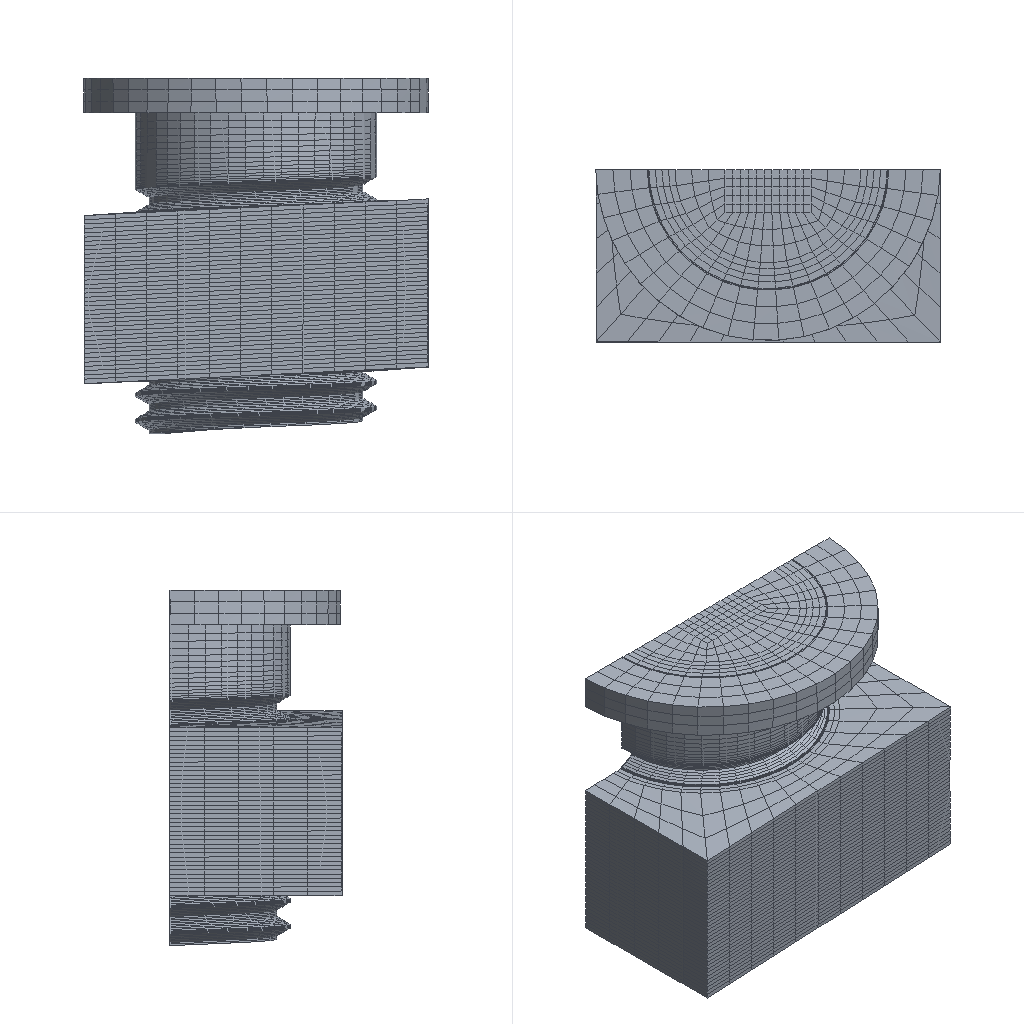Simulation study | abaqus
Set-up summary:
category,name,step,type,value,unit,region
solver,abaqus,,Abaqus/CAE 2024
units,mm-N-s-tonne (MPa),,inferred,E=213000 density=7.87e-09
analysis,Step-1,,dynamic implicit,time_period=1
mesh,nodes,,,41508
mesh,elements,,,35268
element_type,C3D8I,,,35268
material,MATERIAL-35CRMN,,E,213000
material,MATERIAL-35CRMN,,nu,0.286
material,MATERIAL-35CRMN,,density,7.87e-09
material,MATERIAL-35CRMN,,yield,480
material,MATERIAL-35CRMN,,behaviors,plastic
material,MATERIAL-45,,E,209000
material,MATERIAL-45,,nu,0.269
material,MATERIAL-45,,density,7.85e-09
material,MATERIAL-45,,yield,400
material,MATERIAL-45,,behaviors,plastic
section,MATERIAL-45,,solid section,,,NUT
section,MATERIAL-35CRMN,,solid section,,,BOLT
load,SURFFORCE-1,Step-1,pressure,50,,SUR_ELEMS
bc,Disp-BC-1,Step-1,fixed,[dofs=y],,SET-NODE-SYM-Y
bc,Disp-BC-2,Step-1,fixed,[dofs=rx],,SET-NODE-SYM-Y
bc,Disp-BC-3,Step-1,fixed,[dofs=rz],,SET-NODE-SYM-Y
bc,Disp-BC-4,Step-1,fixed,"[dofs=rx,ry,rz,x,y,z n=6]",,SET-NODE-FIX
contact,INTER1-1,initial,contact pair surface to surface,interaction=INTER1; friction=0.15,,SUR_S1 / SUR_M1
Abaqus input file, long lists of numbers shortened:
*Heading
** Job name: deck Model name: Thread
** Generated by: Abaqus/CAE 2024
*Preprint, echo=NO, model=NO, history=NO, contact=NO
**
** PARTS
**
*Part, name=PART-1
*Node
      1,  -6.295, -0.01523,   39.886
      2,  -6.245, -0.01539,    39.75
** (41506 more lines like these left out)
*Element, type=C3D8I
    1,   122,   115,   213,   212,  2308,  2309,  2310,  2311
    2,  2308,  2309,  2310,  2311,  2312,  2313,  2314,  2315
** (35266 more lines like these left out)
*Elset, elset=BOLT, generate
 11194,  35268,      1
*Elset, elset=NUT, generate
     1,  11193,      1
** Section: Section-1-NUT
*Solid Section, elset=NUT, material=MATERIAL-45
,
** Section: Section-2-BOLT
*Solid Section, elset=BOLT, material=MATERIAL-35CRMN
,
*End Part
**
**
** ASSEMBLY
**
*Assembly, name=Assembly
**
*Instance, name=PART-1-1, part=PART-1
*End Instance
**
*Elset, elset=SET-ELEMS, instance=PART-1-1
 26231, 26232, 26234, 26235, 26237, 26238, 26240, 26241, 26243, 26244, 26246, 26247, 26249, 26250, 26252, 26253
 26255, 26256, 26258, 26259, 26261, 26262, 26264, 26265, 26267, 26268, 26270, 26271, 26273, 26274, 26276, 26277
** (6 more lines like these left out)
*Nset, nset=SET-NODE-FIX, instance=PART-1-1
     7,     9,    10,    11,    12,    19,    20,    21,    22,    23,    24,    26,    27,    28,    31,    35
    42,    44,    45,    46,    55,    58,    63,    69,  1067,  1072,  1073,  1077,  1080,  1083,  1085,  1086
** (53 more lines like these left out)
*Nset, nset=SET-NODE-SYM-Y, instance=PART-1-1
     1,     2,     3,     4,    46,    48,    60,    64,    71,    72,    73,    74,    75,    76,    77,    78
    79,    80,    81,    82,    83,    84,    85,    86,    87,    88,    89,    90,    91,    92,    93,    94
** (260 more lines like these left out)
*Elset, elset=_SUR_ELEMS_S3, internal, instance=PART-1-1
 26231, 26232, 26234, 26235, 26237, 26238, 26240, 26241, 26243, 26244, 26246, 26247, 26249, 26250, 26252, 26253
 26255, 26256, 26258, 26259, 26261, 26262, 26264, 26265, 26267, 26268, 26270, 26271, 26273, 26274, 26276, 26277
** (6 more lines like these left out)
*Surface, type=ELEMENT, name=SUR_ELEMS
_SUR_ELEMS_S3, S3
*Elset, elset=_SUR_M1_S3, internal, instance=PART-1-1
 12139, 12140, 12141, 12142, 12143, 12144, 12145, 12146, 12147, 12148, 12149, 12150, 12151, 12152, 12153, 12154
 12155, 12156, 12157, 12158, 12159, 12181, 12182, 12183, 12184, 12185, 12186, 12187, 12188, 12189, 12190, 12191
** (58 more lines like these left out)
*Elset, elset=_SUR_M1_S5, internal, instance=PART-1-1
 12328, 12329, 12330, 12331, 12332, 12333, 12334, 12335, 12336, 12337, 12338, 12339, 12340, 12341, 12342, 12343
 12344, 12345, 12346, 12347, 12348, 12370, 12371, 12372, 12373, 12374, 12375, 12376, 12377, 12378, 12379, 12380
** (46 more lines like these left out)
*Elset, elset=_SUR_M1_S4, internal, instance=PART-1-1
 11656, 11657, 11658, 11659, 11660, 11661, 11662, 11663, 11664, 11665, 11666, 11667, 11668, 11669, 11670, 11671
 11672, 11673, 11674, 11675, 11676, 11698, 11699, 11700, 11701, 11702, 11703, 11704, 11705, 11706, 11707, 11708
** (48 more lines like these left out)
*Elset, elset=_SUR_M1_S6, internal, instance=PART-1-1
 11467, 11468, 11469, 11470, 11471, 11472, 11473, 11474, 11475, 11476, 11477, 11478, 11479, 11480, 11481, 11482
 11483, 11484, 11485, 11486, 11487, 11509, 11510, 11511, 11512, 11513, 11514, 11515, 11516, 11517, 11518, 11519
** (64 more lines like these left out)
*Surface, type=ELEMENT, name=SUR_M1
_SUR_M1_S3, S3
_SUR_M1_S5, S5
_SUR_M1_S4, S4
_SUR_M1_S6, S6
*Elset, elset=_SUR_S1_S3, internal, instance=PART-1-1
    1,    2,    3,    4,    5,    6,    7,    8,    9,   10,   11,   12,   13,   14,   15,   16
   17,   18,   19,   20,   21,   43,   44,   45,   46,   47,   48,   49,   50,   51,   52,   53
** (69 more lines like these left out)
*Elset, elset=_SUR_S1_S6, internal, instance=PART-1-1
  505,  506,  507,  508,  509,  510,  511,  512,  513,  514,  515,  516,  517,  518,  519,  520
  521,  522,  523,  524,  525,  673,  674,  675,  676,  677,  678,  679,  680,  681,  682,  683
** (81 more lines like these left out)
*Surface, type=ELEMENT, name=SUR_S1
_SUR_S1_S3, S3
_SUR_S1_S6, S6
*End Assembly
*Amplitude, name=AMPL-SMOOTH, smooth=0.05
             0.,              0.,              1.,              1.
**
** MATERIALS
**
*Material, name=MATERIAL-35CRMN
*Density
 7.87e-09,
*Elastic
213000., 0.286
*Plastic
 480.,      0.
 500., 0.00282
 580.,   0.012
 680.,   0.045
 850.,    0.11
1000.,     0.3
*Material, name=MATERIAL-45
*Density
 7.85e-09,
*Elastic
209000., 0.269
*Plastic
400.,      0.
420., 0.00152
500.,  0.0295
630.,   0.056
700.,   0.095
760.,    0.25
**
** INTERACTION PROPERTIES
**
*Surface Interaction, name=INTER1
1.,
*Friction, slip tolerance=0.005
 0.15,
**
** INTERACTIONS
**
** Interaction: INTER1-1
*Contact Pair, interaction=INTER1, small sliding, type=SURFACE TO SURFACE, adjust=0.01
SUR_S1, SUR_M1
** ----------------------------------------------------------------
**
** STEP: Step-1
**
*Step, name=Step-1, nlgeom=NO, inc=2000
*Dynamic
0.01,1.,1e-05
**
** BOUNDARY CONDITIONS
**
** Name: Disp-BC-1 Type: Displacement/Rotation
*Boundary
SET-NODE-SYM-Y, 2, 2
** Name: Disp-BC-2 Type: Displacement/Rotation
*Boundary
SET-NODE-SYM-Y, 4, 4
** Name: Disp-BC-3 Type: Displacement/Rotation
*Boundary
SET-NODE-SYM-Y, 6, 6
** Name: Disp-BC-4 Type: Displacement/Rotation
*Boundary
SET-NODE-FIX, 1, 1
SET-NODE-FIX, 2, 2
SET-NODE-FIX, 3, 3
SET-NODE-FIX, 4, 4
SET-NODE-FIX, 5, 5
SET-NODE-FIX, 6, 6
**
** LOADS
**
** Name: SURFFORCE-1   Type: Pressure
*Dsload, amplitude=AMPL-SMOOTH
SUR_ELEMS, P, 50.
**
** OUTPUT REQUESTS
**
*Restart, write, overlay, frequency=5
**
** FIELD OUTPUT: OUTPUT
**
*Output, field, frequency=5
*Contact Output
CDISP, CSTRESS
*Output, history, frequency=0
*End Step
Results summary:
result,odb.job_status,,,JOB_STATUS_COMPLETED_SUCCESSFULLY,"consistent, unstated (Abaqus has no unit system)"
result,steps[0].procedure,Step-1,,*DYNAMIC,"consistent, unstated (Abaqus has no unit system)"
result,steps[0].time_period,Step-1,,1,"consistent, unstated (Abaqus has no unit system)"
result,steps[0].n_frames,Step-1,,4,"consistent, unstated (Abaqus has no unit system)"
result,steps[0].last_frame.id,Step-1,,15,"consistent, unstated (Abaqus has no unit system)"
result,steps[0].last_frame.value,Step-1,,1,"consistent, unstated (Abaqus has no unit system)"
result,steps[0].last_frame.description,Step-1,,Increment     15: Step Time =    1.000,"consistent, unstated (Abaqus has no unit system)"
result,steps[0].completed,Step-1,,True,"consistent, unstated (Abaqus has no unit system)"
result,steps[0].max_U_magnitude,Step-1,,0.06228,"consistent, unstated (Abaqus has no unit system)"
result,steps[0].max_S_mises,Step-1,,613.676,"consistent, unstated (Abaqus has no unit system)"
result,steps[0].diagnostic.n_increments,Step-1,,15,"consistent, unstated (Abaqus has no unit system)"